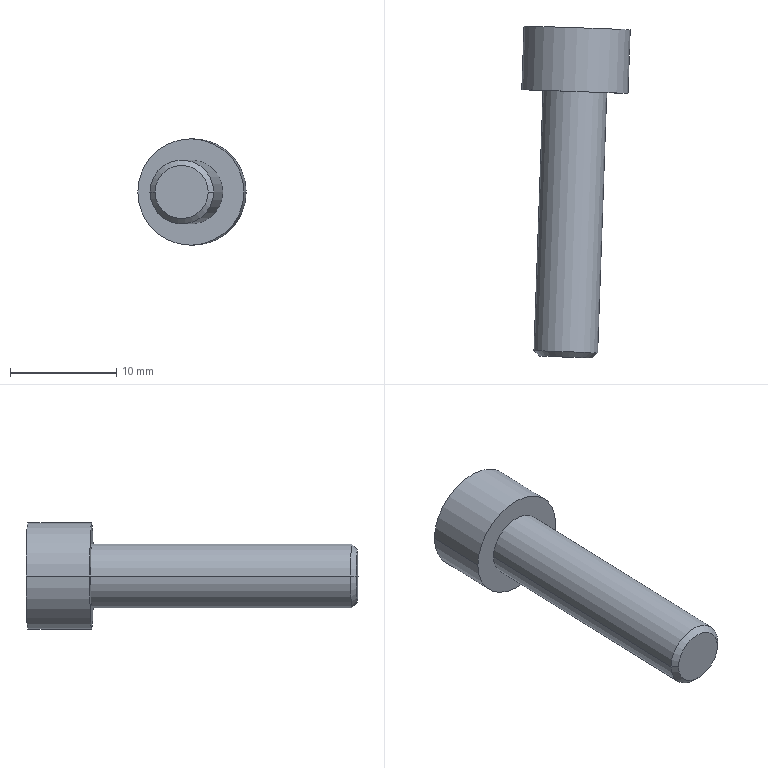Part | STEP file | 1_id1466_x_t | 1 solid | 16 faces | box 10.203 x 31.243 x 10 mm | volume 1111 mm3 | plane 10 | cylinder 4 | cone 2 | commonest cylinder face diameters 6 x2 10 x2
STEP:
#1=CARTESIAN_POINT('',(0.,0.,0.));
#2=DIRECTION('',(0.,0.,1.));
#3=DIRECTION('',(1.,0.,0.));
#4=AXIS2_PLACEMENT_3D('',#1,#2,#3);
#5=CARTESIAN_POINT('',(981.666,161.361,37.96));
#6=VERTEX_POINT('',#5);
#7=CARTESIAN_POINT('',(982.522,185.846,37.96));
#8=VERTEX_POINT('',#7);
#9=CARTESIAN_POINT('',(982.522,185.846,37.96));
#10=DIRECTION('',(0.0349,0.9994,0.));
#11=VECTOR('',#10,1.);
#12=LINE('',#9,#11);
#13=CARTESIAN_POINT('',(979.523,185.951,37.96));
#14=DIRECTION('',(-0.0349,-0.9994,0.));
#15=DIRECTION('',(0.9994,-0.0349,0.));
#16=AXIS2_PLACEMENT_3D('',#13,#14,#15);
#17=CYLINDRICAL_SURFACE('',#16,3.);
#18=CARTESIAN_POINT('',(6.283,0.));
#19=DIRECTION('',(0.,-1.));
#20=VECTOR('',#19,1.);
#21=LINE('',#18,#20);
#22=(GEOMETRIC_REPRESENTATION_CONTEXT(2)PARAMETRIC_REPRESENTATION_CONTEXT()REPRESENTATION_CONTEXT('',''));
#23=DEFINITIONAL_REPRESENTATION('',(#21),#22);
#24=PCURVE('',#17,#23);
#25=CARTESIAN_POINT('',(979.523,185.951,37.96));
#26=DIRECTION('',(-0.0349,-0.9994,0.));
#27=DIRECTION('',(0.9994,-0.0349,0.));
#28=AXIS2_PLACEMENT_3D('',#25,#26,#27);
#29=CYLINDRICAL_SURFACE('',#28,3.);
#30=CARTESIAN_POINT('',(0.,0.));
#31=DIRECTION('',(0.,-1.));
#32=VECTOR('',#31,1.);
#33=LINE('',#30,#32);
#34=(GEOMETRIC_REPRESENTATION_CONTEXT(2)PARAMETRIC_REPRESENTATION_CONTEXT()REPRESENTATION_CONTEXT('',''));
#35=DEFINITIONAL_REPRESENTATION('',(#33),#34);
#36=PCURVE('',#29,#35);
#37=SURFACE_CURVE('',#12,(#24,#36),.PCURVE_S1.);
#38=EDGE_CURVE('',#6,#8,#37,.T.);
#39=ORIENTED_EDGE('',*,*,#38,.F.);
#40=CARTESIAN_POINT('',(975.67,161.571,37.96));
#41=VERTEX_POINT('',#40);
#42=CARTESIAN_POINT('',(978.668,161.466,37.96));
#43=DIRECTION('',(-0.0349,-0.9994,0.));
#44=DIRECTION('',(-0.9994,0.0349,0.));
#45=AXIS2_PLACEMENT_3D('',#42,#43,#44);
#46=CIRCLE('',#45,3.);
#47=CARTESIAN_POINT('',(3.142,24.5));
#48=DIRECTION('',(1.,0.));
#49=VECTOR('',#48,1.);
#50=LINE('',#47,#49);
#51=(GEOMETRIC_REPRESENTATION_CONTEXT(2)PARAMETRIC_REPRESENTATION_CONTEXT()REPRESENTATION_CONTEXT('',''));
#52=DEFINITIONAL_REPRESENTATION('',(#50),#51);
#53=PCURVE('',#17,#52);
#54=CARTESIAN_POINT('',(978.66,161.216,37.96));
#55=DIRECTION('',(0.0349,0.9994,0.));
#56=DIRECTION('',(0.9994,-0.0349,0.));
#57=AXIS2_PLACEMENT_3D('',#54,#55,#56);
#58=CONICAL_SURFACE('',#57,2.75,0.7854);
#59=CARTESIAN_POINT('',(3.142,0.25));
#60=DIRECTION('',(-1.,0.));
#61=VECTOR('',#60,1.);
#62=LINE('',#59,#61);
#63=(GEOMETRIC_REPRESENTATION_CONTEXT(2)PARAMETRIC_REPRESENTATION_CONTEXT()REPRESENTATION_CONTEXT('',''));
#64=DEFINITIONAL_REPRESENTATION('',(#62),#63);
#65=PCURVE('',#58,#64);
#66=SURFACE_CURVE('',#46,(#53,#65),.PCURVE_S1.);
#67=EDGE_CURVE('',#41,#6,#66,.T.);
#68=ORIENTED_EDGE('',*,*,#67,.F.);
#69=CARTESIAN_POINT('',(976.525,186.056,37.96));
#70=VERTEX_POINT('',#69);
#71=CARTESIAN_POINT('',(976.525,186.056,37.96));
#72=DIRECTION('',(-0.0349,-0.9994,0.));
#73=VECTOR('',#72,1.);
#74=LINE('',#71,#73);
#75=CARTESIAN_POINT('',(3.142,0.));
#76=DIRECTION('',(0.,1.));
#77=VECTOR('',#76,1.);
#78=LINE('',#75,#77);
#79=(GEOMETRIC_REPRESENTATION_CONTEXT(2)PARAMETRIC_REPRESENTATION_CONTEXT()REPRESENTATION_CONTEXT('',''));
#80=DEFINITIONAL_REPRESENTATION('',(#78),#79);
#81=PCURVE('',#17,#80);
#82=CARTESIAN_POINT('',(3.142,0.));
#83=DIRECTION('',(0.,1.));
#84=VECTOR('',#83,1.);
#85=LINE('',#82,#84);
#86=(GEOMETRIC_REPRESENTATION_CONTEXT(2)PARAMETRIC_REPRESENTATION_CONTEXT()REPRESENTATION_CONTEXT('',''));
#87=DEFINITIONAL_REPRESENTATION('',(#85),#86);
#88=PCURVE('',#29,#87);
#89=SURFACE_CURVE('',#74,(#81,#88),.PCURVE_S1.);
#90=EDGE_CURVE('',#70,#41,#89,.T.);
#91=ORIENTED_EDGE('',*,*,#90,.F.);
#92=CARTESIAN_POINT('',(979.523,185.951,37.96));
#93=DIRECTION('',(0.0349,0.9994,0.));
#94=DIRECTION('',(0.9994,-0.0349,0.));
#95=AXIS2_PLACEMENT_3D('',#92,#93,#94);
#96=CIRCLE('',#95,3.);
#97=CARTESIAN_POINT('',(6.283,0.));
#98=DIRECTION('',(-1.,0.));
#99=VECTOR('',#98,1.);
#100=LINE('',#97,#99);
#101=(GEOMETRIC_REPRESENTATION_CONTEXT(2)PARAMETRIC_REPRESENTATION_CONTEXT()REPRESENTATION_CONTEXT('',''));
#102=DEFINITIONAL_REPRESENTATION('',(#100),#101);
#103=PCURVE('',#17,#102);
#104=CARTESIAN_POINT('',(979.523,185.951,32.96));
#105=DIRECTION('',(-0.0349,-0.9994,0.));
#106=DIRECTION('',(0.,0.,1.));
#107=AXIS2_PLACEMENT_3D('',#104,#105,#106);
#108=PLANE('',#107);
#109=CARTESIAN_POINT('',(5.,-3.));
#110=CARTESIAN_POINT('',(-0.1962,-3.));
#111=CARTESIAN_POINT('',(2.402,1.5));
#112=CARTESIAN_POINT('',(5.,6.));
#113=CARTESIAN_POINT('',(7.598,1.5));
#114=CARTESIAN_POINT('',(10.196,-3.));
#115=CARTESIAN_POINT('',(5.,-3.));
#116=(BOUNDED_CURVE()B_SPLINE_CURVE(2,(#109,#110,#111,#112,#113,#114,#115),.UNSPECIFIED.,.T.,.F.)B_SPLINE_CURVE_WITH_KNOTS((1,2,2,2,2,1),(-2.094,0.,2.094,4.189,6.283,8.378),.UNSPECIFIED.)CURVE()GEOMETRIC_REPRESENTATION_ITEM()RATIONAL_B_SPLINE_CURVE((1.,0.5,1.,0.5,1.,0.5,1.))REPRESENTATION_ITEM(''));
#117=(GEOMETRIC_REPRESENTATION_CONTEXT(2)PARAMETRIC_REPRESENTATION_CONTEXT()REPRESENTATION_CONTEXT('',''));
#118=DEFINITIONAL_REPRESENTATION('',(#116),#117);
#119=PCURVE('',#108,#118);
#120=SURFACE_CURVE('',#96,(#103,#119),.PCURVE_S1.);
#121=EDGE_CURVE('',#8,#70,#120,.T.);
#122=ORIENTED_EDGE('',*,*,#121,.F.);
#123=EDGE_LOOP('',(#39,#68,#91,#122));
#124=FACE_BOUND('',#123,.T.);
#125=ADVANCED_FACE('',(#124),#17,.T.);
#126=CARTESIAN_POINT('',(984.52,185.777,37.96));
#127=VERTEX_POINT('',#126);
#128=CARTESIAN_POINT('',(974.526,186.126,37.96));
#129=VERTEX_POINT('',#128);
#130=CARTESIAN_POINT('',(979.523,185.951,37.96));
#131=DIRECTION('',(-0.0349,-0.9994,0.));
#132=DIRECTION('',(0.9994,-0.0349,0.));
#133=AXIS2_PLACEMENT_3D('',#130,#131,#132);
#134=CIRCLE('',#133,5.);
#135=CARTESIAN_POINT('',(5.,0.));
#136=DIRECTION('',(0.,-1.));
#137=AXIS2_PLACEMENT_2D('',#135,#136);
#138=CIRCLE('',#137,5.);
#139=(GEOMETRIC_REPRESENTATION_CONTEXT(2)PARAMETRIC_REPRESENTATION_CONTEXT()REPRESENTATION_CONTEXT('',''));
#140=DEFINITIONAL_REPRESENTATION('',(#138),#139);
#141=PCURVE('',#108,#140);
#142=CARTESIAN_POINT('',(979.523,185.951,37.96));
#143=DIRECTION('',(-0.0349,-0.9994,0.));
#144=DIRECTION('',(0.9994,-0.0349,0.));
#145=AXIS2_PLACEMENT_3D('',#142,#143,#144);
#146=CYLINDRICAL_SURFACE('',#145,5.);
#147=CARTESIAN_POINT('',(0.,0.));
#148=DIRECTION('',(1.,0.));
#149=VECTOR('',#148,1.);
#150=LINE('',#147,#149);
#151=(GEOMETRIC_REPRESENTATION_CONTEXT(2)PARAMETRIC_REPRESENTATION_CONTEXT()REPRESENTATION_CONTEXT('',''));
#152=DEFINITIONAL_REPRESENTATION('',(#150),#151);
#153=PCURVE('',#146,#152);
#154=SURFACE_CURVE('',#134,(#141,#153),.PCURVE_S1.);
#155=EDGE_CURVE('',#127,#129,#154,.T.);
#156=ORIENTED_EDGE('',*,*,#155,.T.);
#157=CARTESIAN_POINT('',(979.523,185.951,37.96));
#158=DIRECTION('',(-0.0349,-0.9994,0.));
#159=DIRECTION('',(-0.9994,0.0349,0.));
#160=AXIS2_PLACEMENT_3D('',#157,#158,#159);
#161=CIRCLE('',#160,5.);
#162=CARTESIAN_POINT('',(5.,0.));
#163=DIRECTION('',(0.,1.));
#164=AXIS2_PLACEMENT_2D('',#162,#163);
#165=CIRCLE('',#164,5.);
#166=(GEOMETRIC_REPRESENTATION_CONTEXT(2)PARAMETRIC_REPRESENTATION_CONTEXT()REPRESENTATION_CONTEXT('',''));
#167=DEFINITIONAL_REPRESENTATION('',(#165),#166);
#168=PCURVE('',#108,#167);
#169=CARTESIAN_POINT('',(979.523,185.951,37.96));
#170=DIRECTION('',(-0.0349,-0.9994,0.));
#171=DIRECTION('',(0.9994,-0.0349,0.));
#172=AXIS2_PLACEMENT_3D('',#169,#170,#171);
#173=CYLINDRICAL_SURFACE('',#172,5.);
#174=CARTESIAN_POINT('',(3.142,0.));
#175=DIRECTION('',(1.,0.));
#176=VECTOR('',#175,1.);
#177=LINE('',#174,#176);
#178=(GEOMETRIC_REPRESENTATION_CONTEXT(2)PARAMETRIC_REPRESENTATION_CONTEXT()REPRESENTATION_CONTEXT('',''));
#179=DEFINITIONAL_REPRESENTATION('',(#177),#178);
#180=PCURVE('',#173,#179);
#181=SURFACE_CURVE('',#161,(#168,#180),.PCURVE_S1.);
#182=EDGE_CURVE('',#129,#127,#181,.T.);
#183=ORIENTED_EDGE('',*,*,#182,.T.);
#184=EDGE_LOOP('',(#156,#183));
#185=FACE_BOUND('',#184,.T.);
#186=ORIENTED_EDGE('',*,*,#121,.T.);
#187=CARTESIAN_POINT('',(979.523,185.951,37.96));
#188=DIRECTION('',(0.0349,0.9994,0.));
#189=DIRECTION('',(-0.9994,0.0349,0.));
#190=AXIS2_PLACEMENT_3D('',#187,#188,#189);
#191=CIRCLE('',#190,3.);
#192=CARTESIAN_POINT('',(5.,3.));
#193=CARTESIAN_POINT('',(10.196,3.));
#194=CARTESIAN_POINT('',(7.598,-1.5));
#195=CARTESIAN_POINT('',(5.,-6.));
#196=CARTESIAN_POINT('',(2.402,-1.5));
#197=CARTESIAN_POINT('',(-0.1962,3.));
#198=CARTESIAN_POINT('',(5.,3.));
#199=(BOUNDED_CURVE()B_SPLINE_CURVE(2,(#192,#193,#194,#195,#196,#197,#198),.UNSPECIFIED.,.T.,.F.)B_SPLINE_CURVE_WITH_KNOTS((1,2,2,2,2,1),(-2.094,0.,2.094,4.189,6.283,8.378),.UNSPECIFIED.)CURVE()GEOMETRIC_REPRESENTATION_ITEM()RATIONAL_B_SPLINE_CURVE((1.,0.5,1.,0.5,1.,0.5,1.))REPRESENTATION_ITEM(''));
#200=(GEOMETRIC_REPRESENTATION_CONTEXT(2)PARAMETRIC_REPRESENTATION_CONTEXT()REPRESENTATION_CONTEXT('',''));
#201=DEFINITIONAL_REPRESENTATION('',(#199),#200);
#202=PCURVE('',#108,#201);
#203=CARTESIAN_POINT('',(3.142,0.));
#204=DIRECTION('',(-1.,0.));
#205=VECTOR('',#204,1.);
#206=LINE('',#203,#205);
#207=(GEOMETRIC_REPRESENTATION_CONTEXT(2)PARAMETRIC_REPRESENTATION_CONTEXT()REPRESENTATION_CONTEXT('',''));
#208=DEFINITIONAL_REPRESENTATION('',(#206),#207);
#209=PCURVE('',#29,#208);
#210=SURFACE_CURVE('',#191,(#202,#209),.PCURVE_S1.);
#211=EDGE_CURVE('',#70,#8,#210,.T.);
#212=ORIENTED_EDGE('',*,*,#211,.T.);
#213=EDGE_LOOP('',(#186,#212));
#214=FACE_BOUND('',#213,.T.);
#215=ADVANCED_FACE('',(#185,#214),#108,.T.);
#216=CARTESIAN_POINT('',(984.73,191.773,37.96));
#217=VERTEX_POINT('',#216);
#218=CARTESIAN_POINT('',(984.73,191.773,37.96));
#219=DIRECTION('',(0.0349,0.9994,0.));
#220=VECTOR('',#219,1.);
#221=LINE('',#218,#220);
#222=CARTESIAN_POINT('',(6.283,-6.));
#223=DIRECTION('',(0.,-1.));
#224=VECTOR('',#223,1.);
#225=LINE('',#222,#224);
#226=(GEOMETRIC_REPRESENTATION_CONTEXT(2)PARAMETRIC_REPRESENTATION_CONTEXT()REPRESENTATION_CONTEXT('',''));
#227=DEFINITIONAL_REPRESENTATION('',(#225),#226);
#228=PCURVE('',#173,#227);
#229=CARTESIAN_POINT('',(0.,-6.));
#230=DIRECTION('',(0.,-1.));
#231=VECTOR('',#230,1.);
#232=LINE('',#229,#231);
#233=(GEOMETRIC_REPRESENTATION_CONTEXT(2)PARAMETRIC_REPRESENTATION_CONTEXT()REPRESENTATION_CONTEXT('',''));
#234=DEFINITIONAL_REPRESENTATION('',(#232),#233);
#235=PCURVE('',#146,#234);
#236=SURFACE_CURVE('',#221,(#228,#235),.PCURVE_S1.);
#237=EDGE_CURVE('',#127,#217,#236,.T.);
#238=ORIENTED_EDGE('',*,*,#237,.F.);
#239=ORIENTED_EDGE('',*,*,#182,.F.);
#240=CARTESIAN_POINT('',(974.736,192.122,37.96));
#241=VERTEX_POINT('',#240);
#242=CARTESIAN_POINT('',(974.736,192.122,37.96));
#243=DIRECTION('',(-0.0349,-0.9994,0.));
#244=VECTOR('',#243,1.);
#245=LINE('',#242,#244);
#246=CARTESIAN_POINT('',(3.142,-6.));
#247=DIRECTION('',(0.,1.));
#248=VECTOR('',#247,1.);
#249=LINE('',#246,#248);
#250=(GEOMETRIC_REPRESENTATION_CONTEXT(2)PARAMETRIC_REPRESENTATION_CONTEXT()REPRESENTATION_CONTEXT('',''));
#251=DEFINITIONAL_REPRESENTATION('',(#249),#250);
#252=PCURVE('',#173,#251);
#253=CARTESIAN_POINT('',(3.142,-6.));
#254=DIRECTION('',(0.,1.));
#255=VECTOR('',#254,1.);
#256=LINE('',#253,#255);
#257=(GEOMETRIC_REPRESENTATION_CONTEXT(2)PARAMETRIC_REPRESENTATION_CONTEXT()REPRESENTATION_CONTEXT('',''));
#258=DEFINITIONAL_REPRESENTATION('',(#256),#257);
#259=PCURVE('',#146,#258);
#260=SURFACE_CURVE('',#245,(#252,#259),.PCURVE_S1.);
#261=EDGE_CURVE('',#241,#129,#260,.T.);
#262=ORIENTED_EDGE('',*,*,#261,.F.);
#263=CARTESIAN_POINT('',(979.733,191.948,37.96));
#264=DIRECTION('',(0.0349,0.9994,0.));
#265=DIRECTION('',(0.9994,-0.0349,0.));
#266=AXIS2_PLACEMENT_3D('',#263,#264,#265);
#267=CIRCLE('',#266,5.);
#268=CARTESIAN_POINT('',(6.283,-6.));
#269=DIRECTION('',(-1.,0.));
#270=VECTOR('',#269,1.);
#271=LINE('',#268,#270);
#272=(GEOMETRIC_REPRESENTATION_CONTEXT(2)PARAMETRIC_REPRESENTATION_CONTEXT()REPRESENTATION_CONTEXT('',''));
#273=DEFINITIONAL_REPRESENTATION('',(#271),#272);
#274=PCURVE('',#173,#273);
#275=CARTESIAN_POINT('',(979.733,191.948,37.96));
#276=DIRECTION('',(0.0349,0.9994,0.));
#277=DIRECTION('',(0.,0.,-1.));
#278=AXIS2_PLACEMENT_3D('',#275,#276,#277);
#279=PLANE('',#278);
#280=CARTESIAN_POINT('',(0.,0.));
#281=DIRECTION('',(0.,-1.));
#282=AXIS2_PLACEMENT_2D('',#280,#281);
#283=CIRCLE('',#282,5.);
#284=(GEOMETRIC_REPRESENTATION_CONTEXT(2)PARAMETRIC_REPRESENTATION_CONTEXT()REPRESENTATION_CONTEXT('',''));
#285=DEFINITIONAL_REPRESENTATION('',(#283),#284);
#286=PCURVE('',#279,#285);
#287=SURFACE_CURVE('',#267,(#274,#286),.PCURVE_S1.);
#288=EDGE_CURVE('',#217,#241,#287,.T.);
#289=ORIENTED_EDGE('',*,*,#288,.F.);
#290=EDGE_LOOP('',(#238,#239,#262,#289));
#291=FACE_BOUND('',#290,.T.);
#292=ADVANCED_FACE('',(#291),#173,.T.);
#293=ORIENTED_EDGE('',*,*,#288,.T.);
#294=CARTESIAN_POINT('',(979.733,191.948,37.96));
#295=DIRECTION('',(0.0349,0.9994,0.));
#296=DIRECTION('',(-0.9994,0.0349,0.));
#297=AXIS2_PLACEMENT_3D('',#294,#295,#296);
#298=CIRCLE('',#297,5.);
#299=CARTESIAN_POINT('',(0.,0.));
#300=DIRECTION('',(0.,1.));
#301=AXIS2_PLACEMENT_2D('',#299,#300);
#302=CIRCLE('',#301,5.);
#303=(GEOMETRIC_REPRESENTATION_CONTEXT(2)PARAMETRIC_REPRESENTATION_CONTEXT()REPRESENTATION_CONTEXT('',''));
#304=DEFINITIONAL_REPRESENTATION('',(#302),#303);
#305=PCURVE('',#279,#304);
#306=CARTESIAN_POINT('',(3.142,-6.));
#307=DIRECTION('',(-1.,0.));
#308=VECTOR('',#307,1.);
#309=LINE('',#306,#308);
#310=(GEOMETRIC_REPRESENTATION_CONTEXT(2)PARAMETRIC_REPRESENTATION_CONTEXT()REPRESENTATION_CONTEXT('',''));
#311=DEFINITIONAL_REPRESENTATION('',(#309),#310);
#312=PCURVE('',#146,#311);
#313=SURFACE_CURVE('',#298,(#305,#312),.PCURVE_S1.);
#314=EDGE_CURVE('',#241,#217,#313,.T.);
#315=ORIENTED_EDGE('',*,*,#314,.T.);
#316=EDGE_LOOP('',(#293,#315));
#317=FACE_BOUND('',#316,.T.);
#318=CARTESIAN_POINT('',(976.848,192.048,37.96));
#319=VERTEX_POINT('',#318);
#320=CARTESIAN_POINT('',(978.29,191.998,35.46));
#321=VERTEX_POINT('',#320);
#322=CARTESIAN_POINT('',(976.848,192.048,37.96));
#323=DIRECTION('',(0.4997,-0.01745,-0.866));
#324=VECTOR('',#323,1.);
#325=LINE('',#322,#324);
#326=CARTESIAN_POINT('',(0.,2.887));
#327=DIRECTION('',(0.866,-0.5));
#328=VECTOR('',#327,1.);
#329=LINE('',#326,#328);
#330=(GEOMETRIC_REPRESENTATION_CONTEXT(2)PARAMETRIC_REPRESENTATION_CONTEXT()REPRESENTATION_CONTEXT('',''));
#331=DEFINITIONAL_REPRESENTATION('',(#329),#330);
#332=PCURVE('',#279,#331);
#333=CARTESIAN_POINT('',(976.952,195.046,37.96));
#334=DIRECTION('',(0.8655,-0.03022,0.5));
#335=DIRECTION('',(-0.0349,-0.9994,0.));
#336=AXIS2_PLACEMENT_3D('',#333,#334,#335);
#337=PLANE('',#336);
#338=CARTESIAN_POINT('',(3.,0.));
#339=DIRECTION('',(0.,1.));
#340=VECTOR('',#339,1.);
#341=LINE('',#338,#340);
#342=(GEOMETRIC_REPRESENTATION_CONTEXT(2)PARAMETRIC_REPRESENTATION_CONTEXT()REPRESENTATION_CONTEXT('',''));
#343=DEFINITIONAL_REPRESENTATION('',(#341),#342);
#344=PCURVE('',#337,#343);
#345=SURFACE_CURVE('',#325,(#332,#344),.PCURVE_S1.);
#346=EDGE_CURVE('',#319,#321,#345,.T.);
#347=ORIENTED_EDGE('',*,*,#346,.T.);
#348=CARTESIAN_POINT('',(981.175,191.897,35.46));
#349=VERTEX_POINT('',#348);
#350=CARTESIAN_POINT('',(981.175,191.897,35.46));
#351=DIRECTION('',(-0.9994,0.0349,0.));
#352=VECTOR('',#351,1.);
#353=LINE('',#350,#352);
#354=CARTESIAN_POINT('',(2.5,-1.443));
#355=DIRECTION('',(0.,1.));
#356=VECTOR('',#355,1.);
#357=LINE('',#354,#356);
#358=(GEOMETRIC_REPRESENTATION_CONTEXT(2)PARAMETRIC_REPRESENTATION_CONTEXT()REPRESENTATION_CONTEXT('',''));
#359=DEFINITIONAL_REPRESENTATION('',(#357),#358);
#360=PCURVE('',#279,#359);
#361=CARTESIAN_POINT('',(978.395,194.996,35.46));
#362=DIRECTION('',(0.,0.,1.));
#363=DIRECTION('',(1.,0.,0.));
#364=AXIS2_PLACEMENT_3D('',#361,#362,#363);
#365=PLANE('',#364);
#366=CARTESIAN_POINT('',(2.78,-3.099));
#367=DIRECTION('',(-0.9994,0.0349));
#368=VECTOR('',#367,1.);
#369=LINE('',#366,#368);
#370=(GEOMETRIC_REPRESENTATION_CONTEXT(2)PARAMETRIC_REPRESENTATION_CONTEXT()REPRESENTATION_CONTEXT('',''));
#371=DEFINITIONAL_REPRESENTATION('',(#369),#370);
#372=PCURVE('',#365,#371);
#373=SURFACE_CURVE('',#353,(#360,#372),.PCURVE_S1.);
#374=EDGE_CURVE('',#349,#321,#373,.T.);
#375=ORIENTED_EDGE('',*,*,#374,.F.);
#376=CARTESIAN_POINT('',(982.618,191.847,37.96));
#377=VERTEX_POINT('',#376);
#378=CARTESIAN_POINT('',(981.175,191.897,35.46));
#379=DIRECTION('',(0.4997,-0.01745,0.866));
#380=VECTOR('',#379,1.);
#381=LINE('',#378,#380);
#382=CARTESIAN_POINT('',(2.5,-1.443));
#383=DIRECTION('',(-0.866,-0.5));
#384=VECTOR('',#383,1.);
#385=LINE('',#382,#384);
#386=(GEOMETRIC_REPRESENTATION_CONTEXT(2)PARAMETRIC_REPRESENTATION_CONTEXT()REPRESENTATION_CONTEXT('',''));
#387=DEFINITIONAL_REPRESENTATION('',(#385),#386);
#388=PCURVE('',#279,#387);
#389=CARTESIAN_POINT('',(981.28,194.895,35.46));
#390=DIRECTION('',(-0.8655,0.03022,0.5));
#391=DIRECTION('',(0.,0.9982,-0.06034));
#392=AXIS2_PLACEMENT_3D('',#389,#390,#391);
#393=PLANE('',#392);
#394=CARTESIAN_POINT('',(-2.993,0.209));
#395=DIRECTION('',(-0.06967,-0.9976));
#396=VECTOR('',#395,1.);
#397=LINE('',#394,#396);
#398=(GEOMETRIC_REPRESENTATION_CONTEXT(2)PARAMETRIC_REPRESENTATION_CONTEXT()REPRESENTATION_CONTEXT('',''));
#399=DEFINITIONAL_REPRESENTATION('',(#397),#398);
#400=PCURVE('',#393,#399);
#401=SURFACE_CURVE('',#381,(#388,#400),.PCURVE_S1.);
#402=EDGE_CURVE('',#349,#377,#401,.T.);
#403=ORIENTED_EDGE('',*,*,#402,.T.);
#404=CARTESIAN_POINT('',(981.175,191.897,40.46));
#405=VERTEX_POINT('',#404);
#406=CARTESIAN_POINT('',(982.618,191.847,37.96));
#407=DIRECTION('',(-0.4997,0.01745,0.866));
#408=VECTOR('',#407,1.);
#409=LINE('',#406,#408);
#410=CARTESIAN_POINT('',(0.,-2.887));
#411=DIRECTION('',(-0.866,0.5));
#412=VECTOR('',#411,1.);
#413=LINE('',#410,#412);
#414=(GEOMETRIC_REPRESENTATION_CONTEXT(2)PARAMETRIC_REPRESENTATION_CONTEXT()REPRESENTATION_CONTEXT('',''));
#415=DEFINITIONAL_REPRESENTATION('',(#413),#414);
#416=PCURVE('',#279,#415);
#417=CARTESIAN_POINT('',(982.722,194.845,37.96));
#418=DIRECTION('',(-0.8655,0.03022,-0.5));
#419=DIRECTION('',(0.,0.9982,0.06034));
#420=AXIS2_PLACEMENT_3D('',#417,#418,#419);
#421=PLANE('',#420);
#422=CARTESIAN_POINT('',(-2.993,-0.209));
#423=DIRECTION('',(0.06967,-0.9976));
#424=VECTOR('',#423,1.);
#425=LINE('',#422,#424);
#426=(GEOMETRIC_REPRESENTATION_CONTEXT(2)PARAMETRIC_REPRESENTATION_CONTEXT()REPRESENTATION_CONTEXT('',''));
#427=DEFINITIONAL_REPRESENTATION('',(#425),#426);
#428=PCURVE('',#421,#427);
#429=SURFACE_CURVE('',#409,(#416,#428),.PCURVE_S1.);
#430=EDGE_CURVE('',#377,#405,#429,.T.);
#431=ORIENTED_EDGE('',*,*,#430,.T.);
#432=CARTESIAN_POINT('',(978.29,191.998,40.46));
#433=VERTEX_POINT('',#432);
#434=CARTESIAN_POINT('',(978.29,191.998,40.46));
#435=DIRECTION('',(0.9994,-0.0349,0.));
#436=VECTOR('',#435,1.);
#437=LINE('',#434,#436);
#438=CARTESIAN_POINT('',(-2.5,1.443));
#439=DIRECTION('',(0.,-1.));
#440=VECTOR('',#439,1.);
#441=LINE('',#438,#440);
#442=(GEOMETRIC_REPRESENTATION_CONTEXT(2)PARAMETRIC_REPRESENTATION_CONTEXT()REPRESENTATION_CONTEXT('',''));
#443=DEFINITIONAL_REPRESENTATION('',(#441),#442);
#444=PCURVE('',#279,#443);
#445=CARTESIAN_POINT('',(981.28,194.895,40.46));
#446=DIRECTION('',(0.,0.,-1.));
#447=DIRECTION('',(0.,1.,0.));
#448=AXIS2_PLACEMENT_3D('',#445,#446,#447);
#449=PLANE('',#448);
#450=CARTESIAN_POINT('',(-2.897,-2.99));
#451=DIRECTION('',(-0.0349,0.9994));
#452=VECTOR('',#451,1.);
#453=LINE('',#450,#452);
#454=(GEOMETRIC_REPRESENTATION_CONTEXT(2)PARAMETRIC_REPRESENTATION_CONTEXT()REPRESENTATION_CONTEXT('',''));
#455=DEFINITIONAL_REPRESENTATION('',(#453),#454);
#456=PCURVE('',#449,#455);
#457=SURFACE_CURVE('',#437,(#444,#456),.PCURVE_S1.);
#458=EDGE_CURVE('',#433,#405,#457,.T.);
#459=ORIENTED_EDGE('',*,*,#458,.F.);
#460=CARTESIAN_POINT('',(978.29,191.998,40.46));
#461=DIRECTION('',(-0.4997,0.01745,-0.866));
#462=VECTOR('',#461,1.);
#463=LINE('',#460,#462);
#464=CARTESIAN_POINT('',(-2.5,1.443));
#465=DIRECTION('',(0.866,0.5));
#466=VECTOR('',#465,1.);
#467=LINE('',#464,#466);
#468=(GEOMETRIC_REPRESENTATION_CONTEXT(2)PARAMETRIC_REPRESENTATION_CONTEXT()REPRESENTATION_CONTEXT('',''));
#469=DEFINITIONAL_REPRESENTATION('',(#467),#468);
#470=PCURVE('',#279,#469);
#471=CARTESIAN_POINT('',(978.395,194.996,40.46));
#472=DIRECTION('',(0.8655,-0.03022,-0.5));
#473=DIRECTION('',(-0.5002,0.,-0.8659));
#474=AXIS2_PLACEMENT_3D('',#471,#472,#473);
#475=PLANE('',#474);
#476=CARTESIAN_POINT('',(0.05237,-3.));
#477=DIRECTION('',(0.9998,0.01746));
#478=VECTOR('',#477,1.);
#479=LINE('',#476,#478);
#480=(GEOMETRIC_REPRESENTATION_CONTEXT(2)PARAMETRIC_REPRESENTATION_CONTEXT()REPRESENTATION_CONTEXT('',''));
#481=DEFINITIONAL_REPRESENTATION('',(#479),#480);
#482=PCURVE('',#475,#481);
#483=SURFACE_CURVE('',#463,(#470,#482),.PCURVE_S1.);
#484=EDGE_CURVE('',#433,#319,#483,.T.);
#485=ORIENTED_EDGE('',*,*,#484,.T.);
#486=EDGE_LOOP('',(#347,#375,#403,#431,#459,#485));
#487=FACE_BOUND('',#486,.T.);
#488=ADVANCED_FACE('',(#317,#487),#279,.T.);
#489=ORIENTED_EDGE('',*,*,#261,.T.);
#490=ORIENTED_EDGE('',*,*,#155,.F.);
#491=ORIENTED_EDGE('',*,*,#237,.T.);
#492=ORIENTED_EDGE('',*,*,#314,.F.);
#493=EDGE_LOOP('',(#489,#490,#491,#492));
#494=FACE_BOUND('',#493,.T.);
#495=ADVANCED_FACE('',(#494),#146,.T.);
#496=ORIENTED_EDGE('',*,*,#484,.F.);
#497=CARTESIAN_POINT('',(978.186,189.,40.46));
#498=VERTEX_POINT('',#497);
#499=CARTESIAN_POINT('',(978.186,189.,40.46));
#500=DIRECTION('',(0.0349,0.9994,0.));
#501=VECTOR('',#500,1.);
#502=LINE('',#499,#501);
#503=CARTESIAN_POINT('',(0.1047,-5.999));
#504=DIRECTION('',(-0.01746,0.9998));
#505=VECTOR('',#504,1.);
#506=LINE('',#503,#505);
#507=(GEOMETRIC_REPRESENTATION_CONTEXT(2)PARAMETRIC_REPRESENTATION_CONTEXT()REPRESENTATION_CONTEXT('',''));
#508=DEFINITIONAL_REPRESENTATION('',(#506),#507);
#509=PCURVE('',#475,#508);
#510=CARTESIAN_POINT('',(-5.896,-3.094));
#511=DIRECTION('',(0.9994,0.0349));
#512=VECTOR('',#511,1.);
#513=LINE('',#510,#512);
#514=(GEOMETRIC_REPRESENTATION_CONTEXT(2)PARAMETRIC_REPRESENTATION_CONTEXT()REPRESENTATION_CONTEXT('',''));
#515=DEFINITIONAL_REPRESENTATION('',(#513),#514);
#516=PCURVE('',#449,#515);
#517=SURFACE_CURVE('',#502,(#509,#516),.PCURVE_S1.);
#518=EDGE_CURVE('',#498,#433,#517,.T.);
#519=ORIENTED_EDGE('',*,*,#518,.F.);
#520=CARTESIAN_POINT('',(976.743,189.05,37.96));
#521=VERTEX_POINT('',#520);
#522=CARTESIAN_POINT('',(976.743,189.05,37.96));
#523=DIRECTION('',(0.4997,-0.01745,0.866));
#524=VECTOR('',#523,1.);
#525=LINE('',#522,#524);
#526=CARTESIAN_POINT('',(2.991,-5.949));
#527=DIRECTION('',(-0.9998,-0.01746));
#528=VECTOR('',#527,1.);
#529=LINE('',#526,#528);
#530=(GEOMETRIC_REPRESENTATION_CONTEXT(2)PARAMETRIC_REPRESENTATION_CONTEXT()REPRESENTATION_CONTEXT('',''));
#531=DEFINITIONAL_REPRESENTATION('',(#529),#530);
#532=PCURVE('',#475,#531);
#533=CARTESIAN_POINT('',(978.186,189.,40.46));
#534=DIRECTION('',(0.0349,0.9994,0.));
#535=DIRECTION('',(0.,0.,-1.));
#536=AXIS2_PLACEMENT_3D('',#533,#534,#535);
#537=PLANE('',#536);
#538=CARTESIAN_POINT('',(2.5,1.443));
#539=DIRECTION('',(-0.866,-0.5));
#540=VECTOR('',#539,1.);
#541=LINE('',#538,#540);
#542=(GEOMETRIC_REPRESENTATION_CONTEXT(2)PARAMETRIC_REPRESENTATION_CONTEXT()REPRESENTATION_CONTEXT('',''));
#543=DEFINITIONAL_REPRESENTATION('',(#541),#542);
#544=PCURVE('',#537,#543);
#545=SURFACE_CURVE('',#525,(#532,#544),.PCURVE_S1.);
#546=EDGE_CURVE('',#521,#498,#545,.T.);
#547=ORIENTED_EDGE('',*,*,#546,.F.);
#548=CARTESIAN_POINT('',(976.743,189.05,37.96));
#549=DIRECTION('',(0.0349,0.9994,0.));
#550=VECTOR('',#549,1.);
#551=LINE('',#548,#550);
#552=CARTESIAN_POINT('',(2.991,-5.949));
#553=DIRECTION('',(-0.01746,0.9998));
#554=VECTOR('',#553,1.);
#555=LINE('',#552,#554);
#556=(GEOMETRIC_REPRESENTATION_CONTEXT(2)PARAMETRIC_REPRESENTATION_CONTEXT()REPRESENTATION_CONTEXT('',''));
#557=DEFINITIONAL_REPRESENTATION('',(#555),#556);
#558=PCURVE('',#475,#557);
#559=CARTESIAN_POINT('',(6.,0.));
#560=DIRECTION('',(-1.,0.));
#561=VECTOR('',#560,1.);
#562=LINE('',#559,#561);
#563=(GEOMETRIC_REPRESENTATION_CONTEXT(2)PARAMETRIC_REPRESENTATION_CONTEXT()REPRESENTATION_CONTEXT('',''));
#564=DEFINITIONAL_REPRESENTATION('',(#562),#563);
#565=PCURVE('',#337,#564);
#566=SURFACE_CURVE('',#551,(#558,#565),.PCURVE_S1.);
#567=EDGE_CURVE('',#521,#319,#566,.T.);
#568=ORIENTED_EDGE('',*,*,#567,.T.);
#569=EDGE_LOOP('',(#496,#519,#547,#568));
#570=FACE_BOUND('',#569,.T.);
#571=ADVANCED_FACE('',(#570),#475,.T.);
#572=ORIENTED_EDGE('',*,*,#346,.F.);
#573=ORIENTED_EDGE('',*,*,#567,.F.);
#574=CARTESIAN_POINT('',(978.186,189.,35.46));
#575=VERTEX_POINT('',#574);
#576=CARTESIAN_POINT('',(978.186,189.,35.46));
#577=DIRECTION('',(-0.4997,0.01745,0.866));
#578=VECTOR('',#577,1.);
#579=LINE('',#576,#578);
#580=CARTESIAN_POINT('',(6.,2.887));
#581=DIRECTION('',(0.,-1.));
#582=VECTOR('',#581,1.);
#583=LINE('',#580,#582);
#584=(GEOMETRIC_REPRESENTATION_CONTEXT(2)PARAMETRIC_REPRESENTATION_CONTEXT()REPRESENTATION_CONTEXT('',''));
#585=DEFINITIONAL_REPRESENTATION('',(#583),#584);
#586=PCURVE('',#337,#585);
#587=CARTESIAN_POINT('',(5.,0.));
#588=DIRECTION('',(-0.866,0.5));
#589=VECTOR('',#588,1.);
#590=LINE('',#587,#589);
#591=(GEOMETRIC_REPRESENTATION_CONTEXT(2)PARAMETRIC_REPRESENTATION_CONTEXT()REPRESENTATION_CONTEXT('',''));
#592=DEFINITIONAL_REPRESENTATION('',(#590),#591);
#593=PCURVE('',#537,#592);
#594=SURFACE_CURVE('',#579,(#586,#593),.PCURVE_S1.);
#595=EDGE_CURVE('',#575,#521,#594,.T.);
#596=ORIENTED_EDGE('',*,*,#595,.F.);
#597=CARTESIAN_POINT('',(978.29,191.998,35.46));
#598=DIRECTION('',(-0.0349,-0.9994,0.));
#599=VECTOR('',#598,1.);
#600=LINE('',#597,#599);
#601=CARTESIAN_POINT('',(3.,2.887));
#602=DIRECTION('',(1.,0.));
#603=VECTOR('',#602,1.);
#604=LINE('',#601,#603);
#605=(GEOMETRIC_REPRESENTATION_CONTEXT(2)PARAMETRIC_REPRESENTATION_CONTEXT()REPRESENTATION_CONTEXT('',''));
#606=DEFINITIONAL_REPRESENTATION('',(#604),#605);
#607=PCURVE('',#337,#606);
#608=CARTESIAN_POINT('',(-0.1047,-2.998));
#609=DIRECTION('',(-0.0349,-0.9994));
#610=VECTOR('',#609,1.);
#611=LINE('',#608,#610);
#612=(GEOMETRIC_REPRESENTATION_CONTEXT(2)PARAMETRIC_REPRESENTATION_CONTEXT()REPRESENTATION_CONTEXT('',''));
#613=DEFINITIONAL_REPRESENTATION('',(#611),#612);
#614=PCURVE('',#365,#613);
#615=SURFACE_CURVE('',#600,(#607,#614),.PCURVE_S1.);
#616=EDGE_CURVE('',#321,#575,#615,.T.);
#617=ORIENTED_EDGE('',*,*,#616,.F.);
#618=EDGE_LOOP('',(#572,#573,#596,#617));
#619=FACE_BOUND('',#618,.T.);
#620=ADVANCED_FACE('',(#619),#337,.T.);
#621=ORIENTED_EDGE('',*,*,#374,.T.);
#622=ORIENTED_EDGE('',*,*,#616,.T.);
#623=CARTESIAN_POINT('',(981.071,188.899,35.46));
#624=VERTEX_POINT('',#623);
#625=CARTESIAN_POINT('',(978.186,189.,35.46));
#626=DIRECTION('',(0.9994,-0.0349,0.));
#627=VECTOR('',#626,1.);
#628=LINE('',#625,#627);
#629=CARTESIAN_POINT('',(-0.2094,-5.996));
#630=DIRECTION('',(0.9994,-0.0349));
#631=VECTOR('',#630,1.);
#632=LINE('',#629,#631);
#633=(GEOMETRIC_REPRESENTATION_CONTEXT(2)PARAMETRIC_REPRESENTATION_CONTEXT()REPRESENTATION_CONTEXT('',''));
#634=DEFINITIONAL_REPRESENTATION('',(#632),#633);
#635=PCURVE('',#365,#634);
#636=CARTESIAN_POINT('',(5.,0.));
#637=DIRECTION('',(0.,-1.));
#638=VECTOR('',#637,1.);
#639=LINE('',#636,#638);
#640=(GEOMETRIC_REPRESENTATION_CONTEXT(2)PARAMETRIC_REPRESENTATION_CONTEXT()REPRESENTATION_CONTEXT('',''));
#641=DEFINITIONAL_REPRESENTATION('',(#639),#640);
#642=PCURVE('',#537,#641);
#643=SURFACE_CURVE('',#628,(#635,#642),.PCURVE_S1.);
#644=EDGE_CURVE('',#575,#624,#643,.T.);
#645=ORIENTED_EDGE('',*,*,#644,.T.);
#646=CARTESIAN_POINT('',(981.071,188.899,35.46));
#647=DIRECTION('',(0.0349,0.9994,0.));
#648=VECTOR('',#647,1.);
#649=LINE('',#646,#648);
#650=CARTESIAN_POINT('',(2.676,-6.097));
#651=DIRECTION('',(0.0349,0.9994));
#652=VECTOR('',#651,1.);
#653=LINE('',#650,#652);
#654=(GEOMETRIC_REPRESENTATION_CONTEXT(2)PARAMETRIC_REPRESENTATION_CONTEXT()REPRESENTATION_CONTEXT('',''));
#655=DEFINITIONAL_REPRESENTATION('',(#653),#654);
#656=PCURVE('',#365,#655);
#657=CARTESIAN_POINT('',(-5.985,0.418));
#658=DIRECTION('',(0.9976,-0.06967));
#659=VECTOR('',#658,1.);
#660=LINE('',#657,#659);
#661=(GEOMETRIC_REPRESENTATION_CONTEXT(2)PARAMETRIC_REPRESENTATION_CONTEXT()REPRESENTATION_CONTEXT('',''));
#662=DEFINITIONAL_REPRESENTATION('',(#660),#661);
#663=PCURVE('',#393,#662);
#664=SURFACE_CURVE('',#649,(#656,#663),.PCURVE_S1.);
#665=EDGE_CURVE('',#624,#349,#664,.T.);
#666=ORIENTED_EDGE('',*,*,#665,.T.);
#667=EDGE_LOOP('',(#621,#622,#645,#666));
#668=FACE_BOUND('',#667,.T.);
#669=ADVANCED_FACE('',(#668),#365,.T.);
#670=ORIENTED_EDGE('',*,*,#402,.F.);
#671=ORIENTED_EDGE('',*,*,#665,.F.);
#672=CARTESIAN_POINT('',(982.513,188.849,37.96));
#673=VERTEX_POINT('',#672);
#674=CARTESIAN_POINT('',(982.513,188.849,37.96));
#675=DIRECTION('',(-0.4997,0.01745,-0.866));
#676=VECTOR('',#675,1.);
#677=LINE('',#674,#676);
#678=CARTESIAN_POINT('',(-6.187,-2.462));
#679=DIRECTION('',(0.06967,0.9976));
#680=VECTOR('',#679,1.);
#681=LINE('',#678,#680);
#682=(GEOMETRIC_REPRESENTATION_CONTEXT(2)PARAMETRIC_REPRESENTATION_CONTEXT()REPRESENTATION_CONTEXT('',''));
#683=DEFINITIONAL_REPRESENTATION('',(#681),#682);
#684=PCURVE('',#393,#683);
#685=CARTESIAN_POINT('',(2.5,-4.33));
#686=DIRECTION('',(0.866,0.5));
#687=VECTOR('',#686,1.);
#688=LINE('',#685,#687);
#689=(GEOMETRIC_REPRESENTATION_CONTEXT(2)PARAMETRIC_REPRESENTATION_CONTEXT()REPRESENTATION_CONTEXT('',''));
#690=DEFINITIONAL_REPRESENTATION('',(#688),#689);
#691=PCURVE('',#537,#690);
#692=SURFACE_CURVE('',#677,(#684,#691),.PCURVE_S1.);
#693=EDGE_CURVE('',#673,#624,#692,.T.);
#694=ORIENTED_EDGE('',*,*,#693,.F.);
#695=CARTESIAN_POINT('',(982.513,188.849,37.96));
#696=DIRECTION('',(0.0349,0.9994,0.));
#697=VECTOR('',#696,1.);
#698=LINE('',#695,#697);
#699=CARTESIAN_POINT('',(-6.187,-2.462));
#700=DIRECTION('',(0.9976,-0.06967));
#701=VECTOR('',#700,1.);
#702=LINE('',#699,#701);
#703=(GEOMETRIC_REPRESENTATION_CONTEXT(2)PARAMETRIC_REPRESENTATION_CONTEXT()REPRESENTATION_CONTEXT('',''));
#704=DEFINITIONAL_REPRESENTATION('',(#702),#703);
#705=PCURVE('',#393,#704);
#706=CARTESIAN_POINT('',(-5.985,-0.418));
#707=DIRECTION('',(0.9976,0.06967));
#708=VECTOR('',#707,1.);
#709=LINE('',#706,#708);
#710=(GEOMETRIC_REPRESENTATION_CONTEXT(2)PARAMETRIC_REPRESENTATION_CONTEXT()REPRESENTATION_CONTEXT('',''));
#711=DEFINITIONAL_REPRESENTATION('',(#709),#710);
#712=PCURVE('',#421,#711);
#713=SURFACE_CURVE('',#698,(#705,#712),.PCURVE_S1.);
#714=EDGE_CURVE('',#673,#377,#713,.T.);
#715=ORIENTED_EDGE('',*,*,#714,.T.);
#716=EDGE_LOOP('',(#670,#671,#694,#715));
#717=FACE_BOUND('',#716,.T.);
#718=ADVANCED_FACE('',(#717),#393,.T.);
#719=ORIENTED_EDGE('',*,*,#430,.F.);
#720=ORIENTED_EDGE('',*,*,#714,.F.);
#721=CARTESIAN_POINT('',(981.071,188.899,40.46));
#722=VERTEX_POINT('',#721);
#723=CARTESIAN_POINT('',(981.071,188.899,40.46));
#724=DIRECTION('',(0.4997,-0.01745,-0.866));
#725=VECTOR('',#724,1.);
#726=LINE('',#723,#725);
#727=CARTESIAN_POINT('',(-5.784,-3.298));
#728=DIRECTION('',(-0.06967,0.9976));
#729=VECTOR('',#728,1.);
#730=LINE('',#727,#729);
#731=(GEOMETRIC_REPRESENTATION_CONTEXT(2)PARAMETRIC_REPRESENTATION_CONTEXT()REPRESENTATION_CONTEXT('',''));
#732=DEFINITIONAL_REPRESENTATION('',(#730),#731);
#733=PCURVE('',#421,#732);
#734=CARTESIAN_POINT('',(0.,-2.887));
#735=DIRECTION('',(0.866,-0.5));
#736=VECTOR('',#735,1.);
#737=LINE('',#734,#736);
#738=(GEOMETRIC_REPRESENTATION_CONTEXT(2)PARAMETRIC_REPRESENTATION_CONTEXT()REPRESENTATION_CONTEXT('',''));
#739=DEFINITIONAL_REPRESENTATION('',(#737),#738);
#740=PCURVE('',#537,#739);
#741=SURFACE_CURVE('',#726,(#733,#740),.PCURVE_S1.);
#742=EDGE_CURVE('',#722,#673,#741,.T.);
#743=ORIENTED_EDGE('',*,*,#742,.F.);
#744=CARTESIAN_POINT('',(981.071,188.899,40.46));
#745=DIRECTION('',(0.0349,0.9994,0.));
#746=VECTOR('',#745,1.);
#747=LINE('',#744,#746);
#748=CARTESIAN_POINT('',(-5.784,-3.298));
#749=DIRECTION('',(0.9976,0.06967));
#750=VECTOR('',#749,1.);
#751=LINE('',#748,#750);
#752=(GEOMETRIC_REPRESENTATION_CONTEXT(2)PARAMETRIC_REPRESENTATION_CONTEXT()REPRESENTATION_CONTEXT('',''));
#753=DEFINITIONAL_REPRESENTATION('',(#751),#752);
#754=PCURVE('',#421,#753);
#755=CARTESIAN_POINT('',(-5.996,-0.2094));
#756=DIRECTION('',(0.9994,0.0349));
#757=VECTOR('',#756,1.);
#758=LINE('',#755,#757);
#759=(GEOMETRIC_REPRESENTATION_CONTEXT(2)PARAMETRIC_REPRESENTATION_CONTEXT()REPRESENTATION_CONTEXT('',''));
#760=DEFINITIONAL_REPRESENTATION('',(#758),#759);
#761=PCURVE('',#449,#760);
#762=SURFACE_CURVE('',#747,(#754,#761),.PCURVE_S1.);
#763=EDGE_CURVE('',#722,#405,#762,.T.);
#764=ORIENTED_EDGE('',*,*,#763,.T.);
#765=EDGE_LOOP('',(#719,#720,#743,#764));
#766=FACE_BOUND('',#765,.T.);
#767=ADVANCED_FACE('',(#766),#421,.T.);
#768=ORIENTED_EDGE('',*,*,#458,.T.);
#769=ORIENTED_EDGE('',*,*,#763,.F.);
#770=CARTESIAN_POINT('',(981.071,188.899,40.46));
#771=DIRECTION('',(-0.9994,0.0349,0.));
#772=VECTOR('',#771,1.);
#773=LINE('',#770,#772);
#774=CARTESIAN_POINT('',(-5.996,-0.2094));
#775=DIRECTION('',(0.0349,-0.9994));
#776=VECTOR('',#775,1.);
#777=LINE('',#774,#776);
#778=(GEOMETRIC_REPRESENTATION_CONTEXT(2)PARAMETRIC_REPRESENTATION_CONTEXT()REPRESENTATION_CONTEXT('',''));
#779=DEFINITIONAL_REPRESENTATION('',(#777),#778);
#780=PCURVE('',#449,#779);
#781=CARTESIAN_POINT('',(0.,-2.887));
#782=DIRECTION('',(0.,1.));
#783=VECTOR('',#782,1.);
#784=LINE('',#781,#783);
#785=(GEOMETRIC_REPRESENTATION_CONTEXT(2)PARAMETRIC_REPRESENTATION_CONTEXT()REPRESENTATION_CONTEXT('',''));
#786=DEFINITIONAL_REPRESENTATION('',(#784),#785);
#787=PCURVE('',#537,#786);
#788=SURFACE_CURVE('',#773,(#780,#787),.PCURVE_S1.);
#789=EDGE_CURVE('',#722,#498,#788,.T.);
#790=ORIENTED_EDGE('',*,*,#789,.T.);
#791=ORIENTED_EDGE('',*,*,#518,.T.);
#792=EDGE_LOOP('',(#768,#769,#790,#791));
#793=FACE_BOUND('',#792,.T.);
#794=ADVANCED_FACE('',(#793),#449,.T.);
#795=ORIENTED_EDGE('',*,*,#742,.T.);
#796=ORIENTED_EDGE('',*,*,#693,.T.);
#797=ORIENTED_EDGE('',*,*,#644,.F.);
#798=ORIENTED_EDGE('',*,*,#595,.T.);
#799=ORIENTED_EDGE('',*,*,#546,.T.);
#800=ORIENTED_EDGE('',*,*,#789,.F.);
#801=EDGE_LOOP('',(#795,#796,#797,#798,#799,#800));
#802=FACE_BOUND('',#801,.T.);
#803=ADVANCED_FACE('',(#802),#537,.T.);
#804=ORIENTED_EDGE('',*,*,#90,.T.);
#805=CARTESIAN_POINT('',(978.668,161.466,37.96));
#806=DIRECTION('',(-0.0349,-0.9994,0.));
#807=DIRECTION('',(0.9994,-0.0349,0.));
#808=AXIS2_PLACEMENT_3D('',#805,#806,#807);
#809=CIRCLE('',#808,3.);
#810=CARTESIAN_POINT('',(0.,24.5));
#811=DIRECTION('',(1.,0.));
#812=VECTOR('',#811,1.);
#813=LINE('',#810,#812);
#814=(GEOMETRIC_REPRESENTATION_CONTEXT(2)PARAMETRIC_REPRESENTATION_CONTEXT()REPRESENTATION_CONTEXT('',''));
#815=DEFINITIONAL_REPRESENTATION('',(#813),#814);
#816=PCURVE('',#29,#815);
#817=CARTESIAN_POINT('',(978.66,161.216,37.96));
#818=DIRECTION('',(0.0349,0.9994,0.));
#819=DIRECTION('',(0.9994,-0.0349,0.));
#820=AXIS2_PLACEMENT_3D('',#817,#818,#819);
#821=CONICAL_SURFACE('',#820,2.75,0.7854);
#822=CARTESIAN_POINT('',(6.283,0.25));
#823=DIRECTION('',(-1.,0.));
#824=VECTOR('',#823,1.);
#825=LINE('',#822,#824);
#826=(GEOMETRIC_REPRESENTATION_CONTEXT(2)PARAMETRIC_REPRESENTATION_CONTEXT()REPRESENTATION_CONTEXT('',''));
#827=DEFINITIONAL_REPRESENTATION('',(#825),#826);
#828=PCURVE('',#821,#827);
#829=SURFACE_CURVE('',#809,(#816,#828),.PCURVE_S1.);
#830=EDGE_CURVE('',#6,#41,#829,.T.);
#831=ORIENTED_EDGE('',*,*,#830,.F.);
#832=ORIENTED_EDGE('',*,*,#38,.T.);
#833=ORIENTED_EDGE('',*,*,#211,.F.);
#834=EDGE_LOOP('',(#804,#831,#832,#833));
#835=FACE_BOUND('',#834,.T.);
#836=ADVANCED_FACE('',(#835),#29,.T.);
#837=CARTESIAN_POINT('',(976.152,161.054,37.96));
#838=VERTEX_POINT('',#837);
#839=CARTESIAN_POINT('',(976.152,161.054,37.96));
#840=DIRECTION('',(0.682,-0.7314,0.));
#841=VECTOR('',#840,1.);
#842=LINE('',#839,#841);
#843=CARTESIAN_POINT('',(3.142,-0.25));
#844=DIRECTION('',(0.,-1.));
#845=VECTOR('',#844,1.);
#846=LINE('',#843,#845);
#847=(GEOMETRIC_REPRESENTATION_CONTEXT(2)PARAMETRIC_REPRESENTATION_CONTEXT()REPRESENTATION_CONTEXT('',''));
#848=DEFINITIONAL_REPRESENTATION('',(#846),#847);
#849=PCURVE('',#821,#848);
#850=CARTESIAN_POINT('',(3.142,-0.25));
#851=DIRECTION('',(0.,-1.));
#852=VECTOR('',#851,1.);
#853=LINE('',#850,#852);
#854=(GEOMETRIC_REPRESENTATION_CONTEXT(2)PARAMETRIC_REPRESENTATION_CONTEXT()REPRESENTATION_CONTEXT('',''));
#855=DEFINITIONAL_REPRESENTATION('',(#853),#854);
#856=PCURVE('',#58,#855);
#857=SURFACE_CURVE('',#842,(#849,#856),.PCURVE_S1.);
#858=EDGE_CURVE('',#41,#838,#857,.T.);
#859=ORIENTED_EDGE('',*,*,#858,.T.);
#860=CARTESIAN_POINT('',(981.149,160.879,37.96));
#861=VERTEX_POINT('',#860);
#862=CARTESIAN_POINT('',(978.651,160.966,37.96));
#863=DIRECTION('',(-0.0349,-0.9994,0.));
#864=DIRECTION('',(0.9994,-0.0349,0.));
#865=AXIS2_PLACEMENT_3D('',#862,#863,#864);
#866=CIRCLE('',#865,2.5);
#867=CARTESIAN_POINT('',(6.283,-0.25));
#868=DIRECTION('',(-1.,0.));
#869=VECTOR('',#868,1.);
#870=LINE('',#867,#869);
#871=(GEOMETRIC_REPRESENTATION_CONTEXT(2)PARAMETRIC_REPRESENTATION_CONTEXT()REPRESENTATION_CONTEXT('',''));
#872=DEFINITIONAL_REPRESENTATION('',(#870),#871);
#873=PCURVE('',#821,#872);
#874=CARTESIAN_POINT('',(978.651,160.966,35.46));
#875=DIRECTION('',(-0.0349,-0.9994,0.));
#876=DIRECTION('',(0.,0.,1.));
#877=AXIS2_PLACEMENT_3D('',#874,#875,#876);
#878=PLANE('',#877);
#879=CARTESIAN_POINT('',(2.5,0.));
#880=DIRECTION('',(0.,-1.));
#881=AXIS2_PLACEMENT_2D('',#879,#880);
#882=CIRCLE('',#881,2.5);
#883=(GEOMETRIC_REPRESENTATION_CONTEXT(2)PARAMETRIC_REPRESENTATION_CONTEXT()REPRESENTATION_CONTEXT('',''));
#884=DEFINITIONAL_REPRESENTATION('',(#882),#883);
#885=PCURVE('',#878,#884);
#886=SURFACE_CURVE('',#866,(#873,#885),.PCURVE_S1.);
#887=EDGE_CURVE('',#861,#838,#886,.T.);
#888=ORIENTED_EDGE('',*,*,#887,.F.);
#889=CARTESIAN_POINT('',(981.149,160.879,37.96));
#890=DIRECTION('',(0.7314,0.682,0.));
#891=VECTOR('',#890,1.);
#892=LINE('',#889,#891);
#893=CARTESIAN_POINT('',(6.283,-0.25));
#894=DIRECTION('',(0.,1.));
#895=VECTOR('',#894,1.);
#896=LINE('',#893,#895);
#897=(GEOMETRIC_REPRESENTATION_CONTEXT(2)PARAMETRIC_REPRESENTATION_CONTEXT()REPRESENTATION_CONTEXT('',''));
#898=DEFINITIONAL_REPRESENTATION('',(#896),#897);
#899=PCURVE('',#821,#898);
#900=CARTESIAN_POINT('',(0.,-0.25));
#901=CARTESIAN_POINT('',(0.,-0.2424));
#902=CARTESIAN_POINT('',(0.,-0.2273));
#903=CARTESIAN_POINT('',(0.,-0.2045));
#904=CARTESIAN_POINT('',(0.,-0.1818));
#905=CARTESIAN_POINT('',(0.,-0.1591));
#906=CARTESIAN_POINT('',(0.,-0.1364));
#907=CARTESIAN_POINT('',(0.,-0.1136));
#908=CARTESIAN_POINT('',(0.,-0.09091));
#909=CARTESIAN_POINT('',(0.,-0.06818));
#910=CARTESIAN_POINT('',(0.,-0.04545));
#911=CARTESIAN_POINT('',(0.,-0.02273));
#912=CARTESIAN_POINT('',(0.,0.));
#913=CARTESIAN_POINT('',(0.,0.02273));
#914=CARTESIAN_POINT('',(0.,0.04545));
#915=CARTESIAN_POINT('',(0.,0.06818));
#916=CARTESIAN_POINT('',(0.,0.09091));
#917=CARTESIAN_POINT('',(0.,0.1136));
#918=CARTESIAN_POINT('',(0.,0.1364));
#919=CARTESIAN_POINT('',(0.,0.1591));
#920=CARTESIAN_POINT('',(0.,0.1818));
#921=CARTESIAN_POINT('',(0.,0.2045));
#922=CARTESIAN_POINT('',(0.,0.2273));
#923=CARTESIAN_POINT('',(0.,0.2424));
#924=CARTESIAN_POINT('',(0.,0.25));
#925=B_SPLINE_CURVE_WITH_KNOTS('',3,(#900,#901,#902,#903,#904,#905,#906,#907,#908,#909,#910,#911,#912,#913,#914,#915,#916,#917,#918,#919,#920,#921,#922,#923,#924),.UNSPECIFIED.,.F.,.F.,(4,1,1,1,1,1,1,1,1,1,1,1,1,1,1,1,1,1,1,1,1,1,4),(0.,0.03214,0.06428,0.09642,0.1286,0.1607,0.1928,0.225,0.2571,0.2893,0.3214,0.3536,0.3857,0.4178,0.45,0.4821,0.5143,0.5464,0.5785,0.6107,0.6428,0.675,0.7071),.QUASI_UNIFORM_KNOTS.);
#926=(GEOMETRIC_REPRESENTATION_CONTEXT(2)PARAMETRIC_REPRESENTATION_CONTEXT()REPRESENTATION_CONTEXT('',''));
#927=DEFINITIONAL_REPRESENTATION('',(#925),#926);
#928=PCURVE('',#58,#927);
#929=SURFACE_CURVE('',#892,(#899,#928),.PCURVE_S1.);
#930=EDGE_CURVE('',#861,#6,#929,.T.);
#931=ORIENTED_EDGE('',*,*,#930,.T.);
#932=ORIENTED_EDGE('',*,*,#830,.T.);
#933=EDGE_LOOP('',(#859,#888,#931,#932));
#934=FACE_BOUND('',#933,.T.);
#935=ADVANCED_FACE('',(#934),#821,.T.);
#936=ORIENTED_EDGE('',*,*,#930,.F.);
#937=CARTESIAN_POINT('',(978.651,160.966,37.96));
#938=DIRECTION('',(-0.0349,-0.9994,0.));
#939=DIRECTION('',(-0.9994,0.0349,0.));
#940=AXIS2_PLACEMENT_3D('',#937,#938,#939);
#941=CIRCLE('',#940,2.5);
#942=CARTESIAN_POINT('',(3.142,-0.25));
#943=DIRECTION('',(-1.,0.));
#944=VECTOR('',#943,1.);
#945=LINE('',#942,#944);
#946=(GEOMETRIC_REPRESENTATION_CONTEXT(2)PARAMETRIC_REPRESENTATION_CONTEXT()REPRESENTATION_CONTEXT('',''));
#947=DEFINITIONAL_REPRESENTATION('',(#945),#946);
#948=PCURVE('',#58,#947);
#949=CARTESIAN_POINT('',(2.5,0.));
#950=DIRECTION('',(0.,1.));
#951=AXIS2_PLACEMENT_2D('',#949,#950);
#952=CIRCLE('',#951,2.5);
#953=(GEOMETRIC_REPRESENTATION_CONTEXT(2)PARAMETRIC_REPRESENTATION_CONTEXT()REPRESENTATION_CONTEXT('',''));
#954=DEFINITIONAL_REPRESENTATION('',(#952),#953);
#955=PCURVE('',#878,#954);
#956=SURFACE_CURVE('',#941,(#948,#955),.PCURVE_S1.);
#957=EDGE_CURVE('',#838,#861,#956,.T.);
#958=ORIENTED_EDGE('',*,*,#957,.F.);
#959=ORIENTED_EDGE('',*,*,#858,.F.);
#960=ORIENTED_EDGE('',*,*,#67,.T.);
#961=EDGE_LOOP('',(#936,#958,#959,#960));
#962=FACE_BOUND('',#961,.T.);
#963=ADVANCED_FACE('',(#962),#58,.T.);
#964=ORIENTED_EDGE('',*,*,#887,.T.);
#965=ORIENTED_EDGE('',*,*,#957,.T.);
#966=EDGE_LOOP('',(#964,#965));
#967=FACE_BOUND('',#966,.T.);
#968=ADVANCED_FACE('',(#967),#878,.T.);
#969=CLOSED_SHELL('',(#125,#215,#292,#488,#495,#571,#620,#669,#718,#767,#794,#803,#836,#935,#963,#968));
#970=MANIFOLD_SOLID_BREP('',#969);
#971=(LENGTH_UNIT()NAMED_UNIT(*)SI_UNIT(.MILLI.,.METRE.));
#972=UNCERTAINTY_MEASURE_WITH_UNIT(LENGTH_MEASURE(0.0000001),#971,'','');
#973=(NAMED_UNIT(*)PLANE_ANGLE_UNIT()SI_UNIT($,.RADIAN.));
#974=(NAMED_UNIT(*)SI_UNIT($,.STERADIAN.)SOLID_ANGLE_UNIT());
#975=(GEOMETRIC_REPRESENTATION_CONTEXT(3)GLOBAL_UNCERTAINTY_ASSIGNED_CONTEXT((#972))GLOBAL_UNIT_ASSIGNED_CONTEXT((#971,#973,#974))REPRESENTATION_CONTEXT('',''));
#976=ADVANCED_BREP_SHAPE_REPRESENTATION('',(#4,#970),#975);